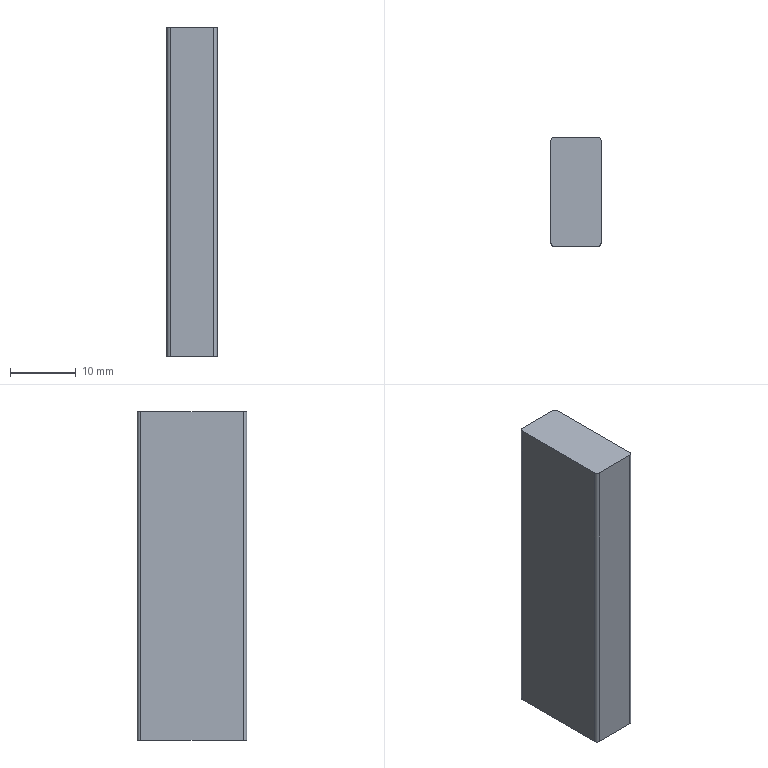Part | NX | features BREP 1 | 1 solid | 10 faces | box 7.6 x 16.6 x 50 mm | volume 6297 mm3 | plane 6 | cylinder 4 | commonest cylinder face diameters 1 x4
STEP:
#1=CARTESIAN_POINT('',(-3.3,8.3,-40.6));
#2=VERTEX_POINT('',#1);
#3=CARTESIAN_POINT('',(-3.8,7.8,-40.6));
#4=VERTEX_POINT('',#3);
#5=CARTESIAN_POINT('',(-3.3,7.8,-40.6));
#6=DIRECTION('',(0.,0.,1.));
#7=DIRECTION('',(1.,0.,0.));
#8=AXIS2_PLACEMENT_3D('',#5,#6,#7);
#9=CIRCLE('',#8,0.5);
#10=EDGE_CURVE('',#2,#4,#9,.T.);
#11=ORIENTED_EDGE('',*,*,#10,.F.);
#12=CARTESIAN_POINT('',(-3.3,8.3,-90.6));
#13=VERTEX_POINT('',#12);
#14=CARTESIAN_POINT('',(-3.3,8.3,-90.6));
#15=DIRECTION('',(0.,0.,1.));
#16=VECTOR('',#15,1000.);
#17=LINE('',#14,#16);
#18=EDGE_CURVE('',#13,#2,#17,.T.);
#19=ORIENTED_EDGE('',*,*,#18,.F.);
#20=CARTESIAN_POINT('',(-3.8,7.8,-90.6));
#21=VERTEX_POINT('',#20);
#22=CARTESIAN_POINT('',(-3.3,7.8,-90.6));
#23=DIRECTION('',(0.,0.,1.));
#24=DIRECTION('',(1.,0.,0.));
#25=AXIS2_PLACEMENT_3D('',#22,#23,#24);
#26=CIRCLE('',#25,0.5);
#27=EDGE_CURVE('',#13,#21,#26,.T.);
#28=ORIENTED_EDGE('',*,*,#27,.T.);
#29=CARTESIAN_POINT('',(-3.8,7.8,-90.6));
#30=DIRECTION('',(0.,0.,1.));
#31=VECTOR('',#30,1000.);
#32=LINE('',#29,#31);
#33=EDGE_CURVE('',#21,#4,#32,.T.);
#34=ORIENTED_EDGE('',*,*,#33,.T.);
#35=EDGE_LOOP('',(#11,#19,#28,#34));
#36=FACE_BOUND('',#35,.T.);
#37=CARTESIAN_POINT('',(-3.3,7.8,-90.6));
#38=DIRECTION('',(0.,0.,1.));
#39=DIRECTION('',(-1.,0.,0.));
#40=AXIS2_PLACEMENT_3D('',#37,#38,#39);
#41=CYLINDRICAL_SURFACE('',#40,0.5);
#42=ADVANCED_FACE('',(#36),#41,.T.);
#43=CARTESIAN_POINT('',(-3.8,-7.8,-40.6));
#44=VERTEX_POINT('',#43);
#45=CARTESIAN_POINT('',(-3.8,-7.8,-40.6));
#46=DIRECTION('',(0.,1.,0.));
#47=VECTOR('',#46,1000.);
#48=LINE('',#45,#47);
#49=EDGE_CURVE('',#44,#4,#48,.T.);
#50=ORIENTED_EDGE('',*,*,#49,.T.);
#51=ORIENTED_EDGE('',*,*,#33,.F.);
#52=CARTESIAN_POINT('',(-3.8,-7.8,-90.6));
#53=VERTEX_POINT('',#52);
#54=CARTESIAN_POINT('',(-3.8,-7.8,-90.6));
#55=DIRECTION('',(0.,1.,0.));
#56=VECTOR('',#55,1000.);
#57=LINE('',#54,#56);
#58=EDGE_CURVE('',#53,#21,#57,.T.);
#59=ORIENTED_EDGE('',*,*,#58,.F.);
#60=CARTESIAN_POINT('',(-3.8,-7.8,-90.6));
#61=DIRECTION('',(0.,0.,1.));
#62=VECTOR('',#61,1000.);
#63=LINE('',#60,#62);
#64=EDGE_CURVE('',#53,#44,#63,.T.);
#65=ORIENTED_EDGE('',*,*,#64,.T.);
#66=EDGE_LOOP('',(#50,#51,#59,#65));
#67=FACE_BOUND('',#66,.T.);
#68=CARTESIAN_POINT('',(-3.8,-7.8,-90.6));
#69=DIRECTION('',(1.,0.,0.));
#70=DIRECTION('',(0.,-1.,0.));
#71=AXIS2_PLACEMENT_3D('',#68,#69,#70);
#72=PLANE('',#71);
#73=ADVANCED_FACE('',(#67),#72,.F.);
#74=CARTESIAN_POINT('',(-3.3,-8.3,-40.6));
#75=VERTEX_POINT('',#74);
#76=CARTESIAN_POINT('',(-3.3,-7.8,-40.6));
#77=DIRECTION('',(0.,0.,1.));
#78=DIRECTION('',(1.,0.,0.));
#79=AXIS2_PLACEMENT_3D('',#76,#77,#78);
#80=CIRCLE('',#79,0.5);
#81=EDGE_CURVE('',#44,#75,#80,.T.);
#82=ORIENTED_EDGE('',*,*,#81,.F.);
#83=ORIENTED_EDGE('',*,*,#64,.F.);
#84=CARTESIAN_POINT('',(-3.3,-8.3,-90.6));
#85=VERTEX_POINT('',#84);
#86=CARTESIAN_POINT('',(-3.3,-7.8,-90.6));
#87=DIRECTION('',(0.,0.,1.));
#88=DIRECTION('',(1.,0.,0.));
#89=AXIS2_PLACEMENT_3D('',#86,#87,#88);
#90=CIRCLE('',#89,0.5);
#91=EDGE_CURVE('',#53,#85,#90,.T.);
#92=ORIENTED_EDGE('',*,*,#91,.T.);
#93=CARTESIAN_POINT('',(-3.3,-8.3,-90.6));
#94=DIRECTION('',(0.,0.,1.));
#95=VECTOR('',#94,1000.);
#96=LINE('',#93,#95);
#97=EDGE_CURVE('',#85,#75,#96,.T.);
#98=ORIENTED_EDGE('',*,*,#97,.T.);
#99=EDGE_LOOP('',(#82,#83,#92,#98));
#100=FACE_BOUND('',#99,.T.);
#101=CARTESIAN_POINT('',(-3.3,-7.8,-90.6));
#102=DIRECTION('',(0.,0.,1.));
#103=DIRECTION('',(-1.,0.,0.));
#104=AXIS2_PLACEMENT_3D('',#101,#102,#103);
#105=CYLINDRICAL_SURFACE('',#104,0.5);
#106=ADVANCED_FACE('',(#100),#105,.T.);
#107=CARTESIAN_POINT('',(3.3,-8.3,-40.6));
#108=VERTEX_POINT('',#107);
#109=CARTESIAN_POINT('',(3.3,-8.3,-40.6));
#110=DIRECTION('',(-1.,0.,0.));
#111=VECTOR('',#110,1000.);
#112=LINE('',#109,#111);
#113=EDGE_CURVE('',#108,#75,#112,.T.);
#114=ORIENTED_EDGE('',*,*,#113,.T.);
#115=ORIENTED_EDGE('',*,*,#97,.F.);
#116=CARTESIAN_POINT('',(3.3,-8.3,-90.6));
#117=VERTEX_POINT('',#116);
#118=CARTESIAN_POINT('',(3.3,-8.3,-90.6));
#119=DIRECTION('',(-1.,0.,0.));
#120=VECTOR('',#119,1000.);
#121=LINE('',#118,#120);
#122=EDGE_CURVE('',#117,#85,#121,.T.);
#123=ORIENTED_EDGE('',*,*,#122,.F.);
#124=CARTESIAN_POINT('',(3.3,-8.3,-90.6));
#125=DIRECTION('',(0.,0.,1.));
#126=VECTOR('',#125,1000.);
#127=LINE('',#124,#126);
#128=EDGE_CURVE('',#117,#108,#127,.T.);
#129=ORIENTED_EDGE('',*,*,#128,.T.);
#130=EDGE_LOOP('',(#114,#115,#123,#129));
#131=FACE_BOUND('',#130,.T.);
#132=CARTESIAN_POINT('',(3.3,-8.3,-90.6));
#133=DIRECTION('',(0.,1.,0.));
#134=DIRECTION('',(0.,0.,-1.));
#135=AXIS2_PLACEMENT_3D('',#132,#133,#134);
#136=PLANE('',#135);
#137=ADVANCED_FACE('',(#131),#136,.F.);
#138=CARTESIAN_POINT('',(3.8,-7.8,-40.6));
#139=VERTEX_POINT('',#138);
#140=CARTESIAN_POINT('',(3.3,-7.8,-40.6));
#141=DIRECTION('',(0.,0.,1.));
#142=DIRECTION('',(1.,0.,0.));
#143=AXIS2_PLACEMENT_3D('',#140,#141,#142);
#144=CIRCLE('',#143,0.5);
#145=EDGE_CURVE('',#108,#139,#144,.T.);
#146=ORIENTED_EDGE('',*,*,#145,.F.);
#147=ORIENTED_EDGE('',*,*,#128,.F.);
#148=CARTESIAN_POINT('',(3.8,-7.8,-90.6));
#149=VERTEX_POINT('',#148);
#150=CARTESIAN_POINT('',(3.3,-7.8,-90.6));
#151=DIRECTION('',(0.,0.,1.));
#152=DIRECTION('',(1.,0.,0.));
#153=AXIS2_PLACEMENT_3D('',#150,#151,#152);
#154=CIRCLE('',#153,0.5);
#155=EDGE_CURVE('',#117,#149,#154,.T.);
#156=ORIENTED_EDGE('',*,*,#155,.T.);
#157=CARTESIAN_POINT('',(3.8,-7.8,-90.6));
#158=DIRECTION('',(0.,0.,1.));
#159=VECTOR('',#158,1000.);
#160=LINE('',#157,#159);
#161=EDGE_CURVE('',#149,#139,#160,.T.);
#162=ORIENTED_EDGE('',*,*,#161,.T.);
#163=EDGE_LOOP('',(#146,#147,#156,#162));
#164=FACE_BOUND('',#163,.T.);
#165=CARTESIAN_POINT('',(3.3,-7.8,-90.6));
#166=DIRECTION('',(0.,0.,1.));
#167=DIRECTION('',(-1.,0.,0.));
#168=AXIS2_PLACEMENT_3D('',#165,#166,#167);
#169=CYLINDRICAL_SURFACE('',#168,0.5);
#170=ADVANCED_FACE('',(#164),#169,.T.);
#171=CARTESIAN_POINT('',(3.8,7.8,-40.6));
#172=VERTEX_POINT('',#171);
#173=CARTESIAN_POINT('',(3.8,7.8,-40.6));
#174=DIRECTION('',(0.,-1.,0.));
#175=VECTOR('',#174,1000.);
#176=LINE('',#173,#175);
#177=EDGE_CURVE('',#172,#139,#176,.T.);
#178=ORIENTED_EDGE('',*,*,#177,.T.);
#179=ORIENTED_EDGE('',*,*,#161,.F.);
#180=CARTESIAN_POINT('',(3.8,7.8,-90.6));
#181=VERTEX_POINT('',#180);
#182=CARTESIAN_POINT('',(3.8,7.8,-90.6));
#183=DIRECTION('',(0.,-1.,0.));
#184=VECTOR('',#183,1000.);
#185=LINE('',#182,#184);
#186=EDGE_CURVE('',#181,#149,#185,.T.);
#187=ORIENTED_EDGE('',*,*,#186,.F.);
#188=CARTESIAN_POINT('',(3.8,7.8,-90.6));
#189=DIRECTION('',(0.,0.,1.));
#190=VECTOR('',#189,1000.);
#191=LINE('',#188,#190);
#192=EDGE_CURVE('',#181,#172,#191,.T.);
#193=ORIENTED_EDGE('',*,*,#192,.T.);
#194=EDGE_LOOP('',(#178,#179,#187,#193));
#195=FACE_BOUND('',#194,.T.);
#196=CARTESIAN_POINT('',(3.8,7.8,-90.6));
#197=DIRECTION('',(-1.,0.,0.));
#198=DIRECTION('',(0.,0.,-1.));
#199=AXIS2_PLACEMENT_3D('',#196,#197,#198);
#200=PLANE('',#199);
#201=ADVANCED_FACE('',(#195),#200,.F.);
#202=CARTESIAN_POINT('',(3.3,8.3,-40.6));
#203=VERTEX_POINT('',#202);
#204=CARTESIAN_POINT('',(3.3,7.8,-40.6));
#205=DIRECTION('',(0.,0.,1.));
#206=DIRECTION('',(1.,0.,0.));
#207=AXIS2_PLACEMENT_3D('',#204,#205,#206);
#208=CIRCLE('',#207,0.5);
#209=EDGE_CURVE('',#172,#203,#208,.T.);
#210=ORIENTED_EDGE('',*,*,#209,.F.);
#211=ORIENTED_EDGE('',*,*,#192,.F.);
#212=CARTESIAN_POINT('',(3.3,8.3,-90.6));
#213=VERTEX_POINT('',#212);
#214=CARTESIAN_POINT('',(3.3,7.8,-90.6));
#215=DIRECTION('',(0.,0.,1.));
#216=DIRECTION('',(1.,0.,0.));
#217=AXIS2_PLACEMENT_3D('',#214,#215,#216);
#218=CIRCLE('',#217,0.5);
#219=EDGE_CURVE('',#181,#213,#218,.T.);
#220=ORIENTED_EDGE('',*,*,#219,.T.);
#221=CARTESIAN_POINT('',(3.3,8.3,-90.6));
#222=DIRECTION('',(0.,0.,1.));
#223=VECTOR('',#222,1000.);
#224=LINE('',#221,#223);
#225=EDGE_CURVE('',#213,#203,#224,.T.);
#226=ORIENTED_EDGE('',*,*,#225,.T.);
#227=EDGE_LOOP('',(#210,#211,#220,#226));
#228=FACE_BOUND('',#227,.T.);
#229=CARTESIAN_POINT('',(3.3,7.8,-90.6));
#230=DIRECTION('',(0.,0.,1.));
#231=DIRECTION('',(-1.,0.,0.));
#232=AXIS2_PLACEMENT_3D('',#229,#230,#231);
#233=CYLINDRICAL_SURFACE('',#232,0.5);
#234=ADVANCED_FACE('',(#228),#233,.T.);
#235=CARTESIAN_POINT('',(-3.3,8.3,-40.6));
#236=DIRECTION('',(1.,0.,0.));
#237=VECTOR('',#236,1000.);
#238=LINE('',#235,#237);
#239=EDGE_CURVE('',#2,#203,#238,.T.);
#240=ORIENTED_EDGE('',*,*,#239,.T.);
#241=ORIENTED_EDGE('',*,*,#225,.F.);
#242=CARTESIAN_POINT('',(-3.3,8.3,-90.6));
#243=DIRECTION('',(1.,0.,0.));
#244=VECTOR('',#243,1000.);
#245=LINE('',#242,#244);
#246=EDGE_CURVE('',#13,#213,#245,.T.);
#247=ORIENTED_EDGE('',*,*,#246,.F.);
#248=ORIENTED_EDGE('',*,*,#18,.T.);
#249=EDGE_LOOP('',(#240,#241,#247,#248));
#250=FACE_BOUND('',#249,.T.);
#251=CARTESIAN_POINT('',(-3.3,8.3,-90.6));
#252=DIRECTION('',(0.,-1.,0.));
#253=DIRECTION('',(-1.,0.,0.));
#254=AXIS2_PLACEMENT_3D('',#251,#252,#253);
#255=PLANE('',#254);
#256=ADVANCED_FACE('',(#250),#255,.F.);
#257=ORIENTED_EDGE('',*,*,#27,.F.);
#258=ORIENTED_EDGE('',*,*,#246,.T.);
#259=ORIENTED_EDGE('',*,*,#219,.F.);
#260=ORIENTED_EDGE('',*,*,#186,.T.);
#261=ORIENTED_EDGE('',*,*,#155,.F.);
#262=ORIENTED_EDGE('',*,*,#122,.T.);
#263=ORIENTED_EDGE('',*,*,#91,.F.);
#264=ORIENTED_EDGE('',*,*,#58,.T.);
#265=EDGE_LOOP('',(#257,#258,#259,#260,#261,#262,#263,#264));
#266=FACE_BOUND('',#265,.T.);
#267=CARTESIAN_POINT('',(-3.3,7.8,-90.6));
#268=DIRECTION('',(0.,0.,1.));
#269=DIRECTION('',(-1.,0.,0.));
#270=AXIS2_PLACEMENT_3D('',#267,#268,#269);
#271=PLANE('',#270);
#272=ADVANCED_FACE('',(#266),#271,.F.);
#273=ORIENTED_EDGE('',*,*,#10,.T.);
#274=ORIENTED_EDGE('',*,*,#49,.F.);
#275=ORIENTED_EDGE('',*,*,#81,.T.);
#276=ORIENTED_EDGE('',*,*,#113,.F.);
#277=ORIENTED_EDGE('',*,*,#145,.T.);
#278=ORIENTED_EDGE('',*,*,#177,.F.);
#279=ORIENTED_EDGE('',*,*,#209,.T.);
#280=ORIENTED_EDGE('',*,*,#239,.F.);
#281=EDGE_LOOP('',(#273,#274,#275,#276,#277,#278,#279,#280));
#282=FACE_BOUND('',#281,.T.);
#283=CARTESIAN_POINT('',(-3.3,7.8,-40.6));
#284=DIRECTION('',(0.,0.,1.));
#285=DIRECTION('',(-1.,0.,0.));
#286=AXIS2_PLACEMENT_3D('',#283,#284,#285);
#287=PLANE('',#286);
#288=ADVANCED_FACE('',(#282),#287,.T.);
#289=CLOSED_SHELL('',(#42,#73,#106,#137,#170,#201,#234,#256,#272,#288));
#290=MANIFOLD_SOLID_BREP('',#289);
#291=(LENGTH_UNIT()NAMED_UNIT(*)SI_UNIT(.MILLI.,.METRE.));
#292=UNCERTAINTY_MEASURE_WITH_UNIT(LENGTH_MEASURE(0.00001),#291,'','');
#293=(NAMED_UNIT(*)PLANE_ANGLE_UNIT()SI_UNIT($,.RADIAN.));
#294=(NAMED_UNIT(*)SI_UNIT($,.STERADIAN.)SOLID_ANGLE_UNIT());
#295=(GEOMETRIC_REPRESENTATION_CONTEXT(3)GLOBAL_UNCERTAINTY_ASSIGNED_CONTEXT((#292))GLOBAL_UNIT_ASSIGNED_CONTEXT((#291,#293,#294))REPRESENTATION_CONTEXT('',''));
#296=ADVANCED_BREP_SHAPE_REPRESENTATION('',(#290),#295);